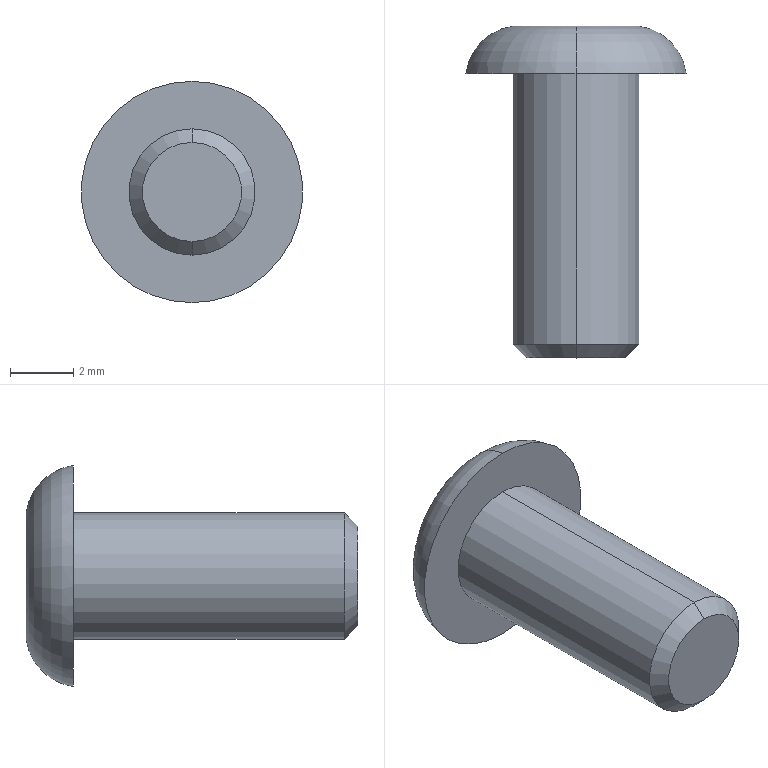Part | SolidWorks | features BaseBody 1 | 1 solid | 16 faces | box 7 x 10.5 x 7 mm | volume 150.453 mm3 | plane 10 | torus 2 | cylinder 2 | cone 2 | commonest cylinder face diameters 4 x2
STEP:
#1=CARTESIAN_POINT('',(17.5,27.,-23.5));
#2=VERTEX_POINT('',#1);
#3=CARTESIAN_POINT('',(17.5,27.,-16.5));
#4=VERTEX_POINT('',#3);
#5=CARTESIAN_POINT('',(17.5,27.,-20.));
#6=DIRECTION('',(0.,-1.,0.));
#7=DIRECTION('',(0.,0.,1.));
#8=AXIS2_PLACEMENT_3D('',#5,#6,#7);
#9=CIRCLE('',#8,3.5);
#10=EDGE_CURVE('',#2,#4,#9,.T.);
#11=ORIENTED_EDGE('',*,*,#10,.F.);
#12=CARTESIAN_POINT('',(17.5,28.5,-22.));
#13=VERTEX_POINT('',#12);
#14=CARTESIAN_POINT('',(17.5,26.766,-21.766));
#15=DIRECTION('',(1.,0.,0.));
#16=DIRECTION('',(0.,0.,-1.));
#17=AXIS2_PLACEMENT_3D('',#14,#15,#16);
#18=CIRCLE('',#17,1.75);
#19=EDGE_CURVE('',#2,#13,#18,.T.);
#20=ORIENTED_EDGE('',*,*,#19,.T.);
#21=CARTESIAN_POINT('',(17.5,28.5,-18.));
#22=VERTEX_POINT('',#21);
#23=CARTESIAN_POINT('',(17.5,28.5,-20.));
#24=DIRECTION('',(0.,-1.,0.));
#25=DIRECTION('',(0.,0.,1.));
#26=AXIS2_PLACEMENT_3D('',#23,#24,#25);
#27=CIRCLE('',#26,2.);
#28=EDGE_CURVE('',#13,#22,#27,.T.);
#29=ORIENTED_EDGE('',*,*,#28,.T.);
#30=CARTESIAN_POINT('',(17.5,26.766,-18.234));
#31=DIRECTION('',(-1.,0.,0.));
#32=DIRECTION('',(0.,-1.,0.));
#33=AXIS2_PLACEMENT_3D('',#30,#31,#32);
#34=CIRCLE('',#33,1.75);
#35=EDGE_CURVE('',#4,#22,#34,.T.);
#36=ORIENTED_EDGE('',*,*,#35,.F.);
#37=EDGE_LOOP('',(#11,#20,#29,#36));
#38=FACE_OUTER_BOUND('',#37,.T.);
#39=CARTESIAN_POINT('',(17.5,26.766,-20.));
#40=DIRECTION('',(0.,1.,0.));
#41=DIRECTION('',(0.,0.,1.));
#42=AXIS2_PLACEMENT_3D('',#39,#40,#41);
#43=TOROIDAL_SURFACE('',#42,1.766,1.75);
#44=ADVANCED_FACE('',(#38),#43,.T.);
#45=CARTESIAN_POINT('',(17.5,27.,-22.));
#46=VERTEX_POINT('',#45);
#47=CARTESIAN_POINT('',(17.5,27.,-18.));
#48=VERTEX_POINT('',#47);
#49=CARTESIAN_POINT('',(17.5,27.,-20.));
#50=DIRECTION('',(0.,-1.,0.));
#51=DIRECTION('',(0.,0.,-1.));
#52=AXIS2_PLACEMENT_3D('',#49,#50,#51);
#53=CIRCLE('',#52,2.);
#54=EDGE_CURVE('',#46,#48,#53,.T.);
#55=ORIENTED_EDGE('',*,*,#54,.T.);
#56=CARTESIAN_POINT('',(17.5,18.43,-18.));
#57=VERTEX_POINT('',#56);
#58=CARTESIAN_POINT('',(17.5,22.715,-18.));
#59=DIRECTION('',(0.,-1.,0.));
#60=VECTOR('',#59,1000.);
#61=LINE('',#58,#60);
#62=EDGE_CURVE('',#48,#57,#61,.T.);
#63=ORIENTED_EDGE('',*,*,#62,.T.);
#64=CARTESIAN_POINT('',(17.5,18.43,-22.));
#65=VERTEX_POINT('',#64);
#66=CARTESIAN_POINT('',(17.5,18.43,-20.));
#67=DIRECTION('',(0.,1.,0.));
#68=DIRECTION('',(0.,0.,-1.));
#69=AXIS2_PLACEMENT_3D('',#66,#67,#68);
#70=CIRCLE('',#69,2.);
#71=EDGE_CURVE('',#57,#65,#70,.T.);
#72=ORIENTED_EDGE('',*,*,#71,.T.);
#73=CARTESIAN_POINT('',(17.5,22.715,-22.));
#74=DIRECTION('',(0.,-1.,0.));
#75=VECTOR('',#74,1000.);
#76=LINE('',#73,#75);
#77=EDGE_CURVE('',#46,#65,#76,.T.);
#78=ORIENTED_EDGE('',*,*,#77,.F.);
#79=EDGE_LOOP('',(#55,#63,#72,#78));
#80=FACE_OUTER_BOUND('',#79,.T.);
#81=CARTESIAN_POINT('',(17.5,22.715,-20.));
#82=DIRECTION('',(0.,-1.,0.));
#83=DIRECTION('',(0.,0.,-1.));
#84=AXIS2_PLACEMENT_3D('',#81,#82,#83);
#85=CYLINDRICAL_SURFACE('',#84,2.);
#86=ADVANCED_FACE('',(#80),#85,.T.);
#87=CARTESIAN_POINT('',(17.5,18.,-18.43));
#88=VERTEX_POINT('',#87);
#89=CARTESIAN_POINT('',(17.5,18.,-21.57));
#90=VERTEX_POINT('',#89);
#91=CARTESIAN_POINT('',(17.5,18.,-20.));
#92=DIRECTION('',(0.,1.,0.));
#93=DIRECTION('',(0.,0.,1.));
#94=AXIS2_PLACEMENT_3D('',#91,#92,#93);
#95=CIRCLE('',#94,1.57);
#96=EDGE_CURVE('',#88,#90,#95,.T.);
#97=ORIENTED_EDGE('',*,*,#96,.T.);
#98=CARTESIAN_POINT('',(17.5,18.43,-22.));
#99=DIRECTION('',(0.,0.7071,-0.7071));
#100=VECTOR('',#99,1000.);
#101=LINE('',#98,#100);
#102=EDGE_CURVE('',#90,#65,#101,.T.);
#103=ORIENTED_EDGE('',*,*,#102,.T.);
#104=ORIENTED_EDGE('',*,*,#71,.F.);
#105=CARTESIAN_POINT('',(17.5,18.43,-18.));
#106=DIRECTION('',(0.,0.7071,0.7071));
#107=VECTOR('',#106,1000.);
#108=LINE('',#105,#107);
#109=EDGE_CURVE('',#88,#57,#108,.T.);
#110=ORIENTED_EDGE('',*,*,#109,.F.);
#111=EDGE_LOOP('',(#97,#103,#104,#110));
#112=FACE_OUTER_BOUND('',#111,.T.);
#113=CARTESIAN_POINT('',(17.5,18.43,-20.));
#114=DIRECTION('',(0.,1.,0.));
#115=DIRECTION('',(0.,0.,1.));
#116=AXIS2_PLACEMENT_3D('',#113,#114,#115);
#117=CONICAL_SURFACE('',#116,2.,0.7854);
#118=ADVANCED_FACE('',(#112),#117,.T.);
#119=CARTESIAN_POINT('',(17.5,27.5,-21.684));
#120=VERTEX_POINT('',#119);
#121=CARTESIAN_POINT('',(16.042,27.5,-20.842));
#122=VERTEX_POINT('',#121);
#123=CARTESIAN_POINT('',(17.5,27.5,-21.684));
#124=DIRECTION('',(-0.866,0.,0.5));
#125=VECTOR('',#124,1000.);
#126=LINE('',#123,#125);
#127=EDGE_CURVE('',#120,#122,#126,.T.);
#128=ORIENTED_EDGE('',*,*,#127,.T.);
#129=CARTESIAN_POINT('',(16.042,27.5,-19.158));
#130=VERTEX_POINT('',#129);
#131=CARTESIAN_POINT('',(16.042,27.5,-20.842));
#132=DIRECTION('',(0.,0.,1.));
#133=VECTOR('',#132,1000.);
#134=LINE('',#131,#133);
#135=EDGE_CURVE('',#122,#130,#134,.T.);
#136=ORIENTED_EDGE('',*,*,#135,.T.);
#137=CARTESIAN_POINT('',(17.5,27.5,-18.316));
#138=VERTEX_POINT('',#137);
#139=CARTESIAN_POINT('',(16.042,27.5,-19.158));
#140=DIRECTION('',(0.866,0.,0.5));
#141=VECTOR('',#140,1000.);
#142=LINE('',#139,#141);
#143=EDGE_CURVE('',#130,#138,#142,.T.);
#144=ORIENTED_EDGE('',*,*,#143,.T.);
#145=CARTESIAN_POINT('',(18.958,27.5,-19.158));
#146=VERTEX_POINT('',#145);
#147=CARTESIAN_POINT('',(17.5,27.5,-18.316));
#148=DIRECTION('',(0.866,0.,-0.5));
#149=VECTOR('',#148,1000.);
#150=LINE('',#147,#149);
#151=EDGE_CURVE('',#138,#146,#150,.T.);
#152=ORIENTED_EDGE('',*,*,#151,.T.);
#153=CARTESIAN_POINT('',(18.958,27.5,-20.842));
#154=VERTEX_POINT('',#153);
#155=CARTESIAN_POINT('',(18.958,27.5,-19.158));
#156=DIRECTION('',(0.,0.,-1.));
#157=VECTOR('',#156,1000.);
#158=LINE('',#155,#157);
#159=EDGE_CURVE('',#146,#154,#158,.T.);
#160=ORIENTED_EDGE('',*,*,#159,.T.);
#161=CARTESIAN_POINT('',(18.958,27.5,-20.842));
#162=DIRECTION('',(-0.866,0.,-0.5));
#163=VECTOR('',#162,1000.);
#164=LINE('',#161,#163);
#165=EDGE_CURVE('',#154,#120,#164,.T.);
#166=ORIENTED_EDGE('',*,*,#165,.T.);
#167=EDGE_LOOP('',(#128,#136,#144,#152,#160,#166));
#168=FACE_OUTER_BOUND('',#167,.T.);
#169=CARTESIAN_POINT('',(17.5,27.5,-20.));
#170=DIRECTION('',(0.,1.,0.));
#171=DIRECTION('',(1.,0.,0.));
#172=AXIS2_PLACEMENT_3D('',#169,#170,#171);
#173=PLANE('',#172);
#174=ADVANCED_FACE('',(#168),#173,.T.);
#175=CARTESIAN_POINT('',(16.042,28.5,-19.158));
#176=VERTEX_POINT('',#175);
#177=CARTESIAN_POINT('',(16.042,28.5,-19.158));
#178=DIRECTION('',(0.,1.,0.));
#179=VECTOR('',#178,1000.);
#180=LINE('',#177,#179);
#181=EDGE_CURVE('',#130,#176,#180,.T.);
#182=ORIENTED_EDGE('',*,*,#181,.T.);
#183=CARTESIAN_POINT('',(17.5,28.5,-18.316));
#184=VERTEX_POINT('',#183);
#185=CARTESIAN_POINT('',(17.5,28.5,-18.316));
#186=DIRECTION('',(-0.866,0.,-0.5));
#187=VECTOR('',#186,1000.);
#188=LINE('',#185,#187);
#189=EDGE_CURVE('',#184,#176,#188,.T.);
#190=ORIENTED_EDGE('',*,*,#189,.F.);
#191=CARTESIAN_POINT('',(17.5,28.5,-18.316));
#192=DIRECTION('',(0.,-1.,0.));
#193=VECTOR('',#192,1000.);
#194=LINE('',#191,#193);
#195=EDGE_CURVE('',#184,#138,#194,.T.);
#196=ORIENTED_EDGE('',*,*,#195,.T.);
#197=ORIENTED_EDGE('',*,*,#143,.F.);
#198=EDGE_LOOP('',(#182,#190,#196,#197));
#199=FACE_OUTER_BOUND('',#198,.T.);
#200=CARTESIAN_POINT('',(16.042,28.5,-19.158));
#201=DIRECTION('',(-0.5,0.,0.866));
#202=DIRECTION('',(0.,1.,0.));
#203=AXIS2_PLACEMENT_3D('',#200,#201,#202);
#204=PLANE('',#203);
#205=ADVANCED_FACE('',(#199),#204,.F.);
#206=CARTESIAN_POINT('',(16.042,28.5,-20.842));
#207=VERTEX_POINT('',#206);
#208=CARTESIAN_POINT('',(16.042,28.5,-20.842));
#209=DIRECTION('',(0.,1.,0.));
#210=VECTOR('',#209,1000.);
#211=LINE('',#208,#210);
#212=EDGE_CURVE('',#122,#207,#211,.T.);
#213=ORIENTED_EDGE('',*,*,#212,.T.);
#214=CARTESIAN_POINT('',(16.042,28.5,-21.));
#215=DIRECTION('',(0.,0.,-1.));
#216=VECTOR('',#215,1000.);
#217=LINE('',#214,#216);
#218=EDGE_CURVE('',#176,#207,#217,.T.);
#219=ORIENTED_EDGE('',*,*,#218,.F.);
#220=ORIENTED_EDGE('',*,*,#181,.F.);
#221=ORIENTED_EDGE('',*,*,#135,.F.);
#222=EDGE_LOOP('',(#213,#219,#220,#221));
#223=FACE_OUTER_BOUND('',#222,.T.);
#224=CARTESIAN_POINT('',(16.042,28.5,-20.842));
#225=DIRECTION('',(-1.,0.,0.));
#226=DIRECTION('',(0.,0.,1.));
#227=AXIS2_PLACEMENT_3D('',#224,#225,#226);
#228=PLANE('',#227);
#229=ADVANCED_FACE('',(#223),#228,.F.);
#230=CARTESIAN_POINT('',(17.5,28.5,-21.684));
#231=VERTEX_POINT('',#230);
#232=CARTESIAN_POINT('',(17.5,28.5,-21.684));
#233=DIRECTION('',(0.,1.,0.));
#234=VECTOR('',#233,1000.);
#235=LINE('',#232,#234);
#236=EDGE_CURVE('',#120,#231,#235,.T.);
#237=ORIENTED_EDGE('',*,*,#236,.T.);
#238=CARTESIAN_POINT('',(16.042,28.5,-20.842));
#239=DIRECTION('',(0.866,0.,-0.5));
#240=VECTOR('',#239,1000.);
#241=LINE('',#238,#240);
#242=EDGE_CURVE('',#207,#231,#241,.T.);
#243=ORIENTED_EDGE('',*,*,#242,.F.);
#244=ORIENTED_EDGE('',*,*,#212,.F.);
#245=ORIENTED_EDGE('',*,*,#127,.F.);
#246=EDGE_LOOP('',(#237,#243,#244,#245));
#247=FACE_OUTER_BOUND('',#246,.T.);
#248=CARTESIAN_POINT('',(17.5,28.5,-21.684));
#249=DIRECTION('',(-0.5,0.,-0.866));
#250=DIRECTION('',(-0.866,0.,0.5));
#251=AXIS2_PLACEMENT_3D('',#248,#249,#250);
#252=PLANE('',#251);
#253=ADVANCED_FACE('',(#247),#252,.F.);
#254=CARTESIAN_POINT('',(18.958,28.5,-20.842));
#255=VERTEX_POINT('',#254);
#256=CARTESIAN_POINT('',(18.958,28.5,-20.842));
#257=DIRECTION('',(0.,1.,0.));
#258=VECTOR('',#257,1000.);
#259=LINE('',#256,#258);
#260=EDGE_CURVE('',#154,#255,#259,.T.);
#261=ORIENTED_EDGE('',*,*,#260,.T.);
#262=CARTESIAN_POINT('',(17.5,28.5,-21.684));
#263=DIRECTION('',(0.866,0.,0.5));
#264=VECTOR('',#263,1000.);
#265=LINE('',#262,#264);
#266=EDGE_CURVE('',#231,#255,#265,.T.);
#267=ORIENTED_EDGE('',*,*,#266,.F.);
#268=ORIENTED_EDGE('',*,*,#236,.F.);
#269=ORIENTED_EDGE('',*,*,#165,.F.);
#270=EDGE_LOOP('',(#261,#267,#268,#269));
#271=FACE_OUTER_BOUND('',#270,.T.);
#272=CARTESIAN_POINT('',(18.958,28.5,-20.842));
#273=DIRECTION('',(0.5,0.,-0.866));
#274=DIRECTION('',(0.,-1.,0.));
#275=AXIS2_PLACEMENT_3D('',#272,#273,#274);
#276=PLANE('',#275);
#277=ADVANCED_FACE('',(#271),#276,.F.);
#278=CARTESIAN_POINT('',(18.958,28.5,-19.158));
#279=VERTEX_POINT('',#278);
#280=CARTESIAN_POINT('',(18.958,28.5,-19.158));
#281=DIRECTION('',(0.,1.,0.));
#282=VECTOR('',#281,1000.);
#283=LINE('',#280,#282);
#284=EDGE_CURVE('',#146,#279,#283,.T.);
#285=ORIENTED_EDGE('',*,*,#284,.T.);
#286=CARTESIAN_POINT('',(18.958,28.5,-21.));
#287=DIRECTION('',(0.,0.,1.));
#288=VECTOR('',#287,1000.);
#289=LINE('',#286,#288);
#290=EDGE_CURVE('',#255,#279,#289,.T.);
#291=ORIENTED_EDGE('',*,*,#290,.F.);
#292=ORIENTED_EDGE('',*,*,#260,.F.);
#293=ORIENTED_EDGE('',*,*,#159,.F.);
#294=EDGE_LOOP('',(#285,#291,#292,#293));
#295=FACE_OUTER_BOUND('',#294,.T.);
#296=CARTESIAN_POINT('',(18.958,28.5,-19.158));
#297=DIRECTION('',(1.,0.,0.));
#298=DIRECTION('',(0.,1.,0.));
#299=AXIS2_PLACEMENT_3D('',#296,#297,#298);
#300=PLANE('',#299);
#301=ADVANCED_FACE('',(#295),#300,.F.);
#302=ORIENTED_EDGE('',*,*,#195,.F.);
#303=CARTESIAN_POINT('',(18.958,28.5,-19.158));
#304=DIRECTION('',(-0.866,0.,0.5));
#305=VECTOR('',#304,1000.);
#306=LINE('',#303,#305);
#307=EDGE_CURVE('',#279,#184,#306,.T.);
#308=ORIENTED_EDGE('',*,*,#307,.F.);
#309=ORIENTED_EDGE('',*,*,#284,.F.);
#310=ORIENTED_EDGE('',*,*,#151,.F.);
#311=EDGE_LOOP('',(#302,#308,#309,#310));
#312=FACE_OUTER_BOUND('',#311,.T.);
#313=CARTESIAN_POINT('',(17.5,28.5,-18.316));
#314=DIRECTION('',(0.5,0.,0.866));
#315=DIRECTION('',(0.,-1.,0.));
#316=AXIS2_PLACEMENT_3D('',#313,#314,#315);
#317=PLANE('',#316);
#318=ADVANCED_FACE('',(#312),#317,.F.);
#319=ORIENTED_EDGE('',*,*,#290,.T.);
#320=ORIENTED_EDGE('',*,*,#307,.T.);
#321=ORIENTED_EDGE('',*,*,#189,.T.);
#322=ORIENTED_EDGE('',*,*,#218,.T.);
#323=ORIENTED_EDGE('',*,*,#242,.T.);
#324=ORIENTED_EDGE('',*,*,#266,.T.);
#325=EDGE_LOOP('',(#319,#320,#321,#322,#323,#324));
#326=FACE_BOUND('',#325,.T.);
#327=CARTESIAN_POINT('',(17.5,28.5,-20.));
#328=DIRECTION('',(0.,-1.,0.));
#329=DIRECTION('',(0.,0.,1.));
#330=AXIS2_PLACEMENT_3D('',#327,#328,#329);
#331=CIRCLE('',#330,2.);
#332=EDGE_CURVE('',#22,#13,#331,.T.);
#333=ORIENTED_EDGE('',*,*,#332,.F.);
#334=ORIENTED_EDGE('',*,*,#28,.F.);
#335=EDGE_LOOP('',(#333,#334));
#336=FACE_OUTER_BOUND('',#335,.T.);
#337=CARTESIAN_POINT('',(17.5,28.5,-21.));
#338=DIRECTION('',(0.,1.,0.));
#339=DIRECTION('',(1.,0.,0.));
#340=AXIS2_PLACEMENT_3D('',#337,#338,#339);
#341=PLANE('',#340);
#342=ADVANCED_FACE('',(#326,#336),#341,.T.);
#343=ORIENTED_EDGE('',*,*,#96,.F.);
#344=CARTESIAN_POINT('',(17.5,18.,-20.));
#345=DIRECTION('',(0.,1.,0.));
#346=DIRECTION('',(0.,0.,1.));
#347=AXIS2_PLACEMENT_3D('',#344,#345,#346);
#348=CIRCLE('',#347,1.57);
#349=EDGE_CURVE('',#90,#88,#348,.T.);
#350=ORIENTED_EDGE('',*,*,#349,.F.);
#351=EDGE_LOOP('',(#343,#350));
#352=FACE_OUTER_BOUND('',#351,.T.);
#353=CARTESIAN_POINT('',(17.5,18.,-20.785));
#354=DIRECTION('',(0.,-1.,0.));
#355=DIRECTION('',(0.,0.,-1.));
#356=AXIS2_PLACEMENT_3D('',#353,#354,#355);
#357=PLANE('',#356);
#358=ADVANCED_FACE('',(#352),#357,.T.);
#359=ORIENTED_EDGE('',*,*,#54,.F.);
#360=CARTESIAN_POINT('',(17.5,27.,-20.));
#361=DIRECTION('',(0.,-1.,0.));
#362=DIRECTION('',(0.,0.,-1.));
#363=AXIS2_PLACEMENT_3D('',#360,#361,#362);
#364=CIRCLE('',#363,2.);
#365=EDGE_CURVE('',#48,#46,#364,.T.);
#366=ORIENTED_EDGE('',*,*,#365,.F.);
#367=EDGE_LOOP('',(#359,#366));
#368=FACE_BOUND('',#367,.T.);
#369=CARTESIAN_POINT('',(17.5,27.,-20.));
#370=DIRECTION('',(0.,-1.,0.));
#371=DIRECTION('',(0.,0.,1.));
#372=AXIS2_PLACEMENT_3D('',#369,#370,#371);
#373=CIRCLE('',#372,3.5);
#374=EDGE_CURVE('',#4,#2,#373,.T.);
#375=ORIENTED_EDGE('',*,*,#374,.T.);
#376=ORIENTED_EDGE('',*,*,#10,.T.);
#377=EDGE_LOOP('',(#375,#376));
#378=FACE_OUTER_BOUND('',#377,.T.);
#379=CARTESIAN_POINT('',(17.5,27.,-22.75));
#380=DIRECTION('',(0.,-1.,0.));
#381=DIRECTION('',(-1.,0.,0.));
#382=AXIS2_PLACEMENT_3D('',#379,#380,#381);
#383=PLANE('',#382);
#384=ADVANCED_FACE('',(#368,#378),#383,.T.);
#385=ORIENTED_EDGE('',*,*,#102,.F.);
#386=ORIENTED_EDGE('',*,*,#349,.T.);
#387=ORIENTED_EDGE('',*,*,#109,.T.);
#388=CARTESIAN_POINT('',(17.5,18.43,-20.));
#389=DIRECTION('',(0.,1.,0.));
#390=DIRECTION('',(0.,0.,-1.));
#391=AXIS2_PLACEMENT_3D('',#388,#389,#390);
#392=CIRCLE('',#391,2.);
#393=EDGE_CURVE('',#65,#57,#392,.T.);
#394=ORIENTED_EDGE('',*,*,#393,.F.);
#395=EDGE_LOOP('',(#385,#386,#387,#394));
#396=FACE_OUTER_BOUND('',#395,.T.);
#397=CARTESIAN_POINT('',(17.5,18.43,-20.));
#398=DIRECTION('',(0.,1.,0.));
#399=DIRECTION('',(0.,0.,1.));
#400=AXIS2_PLACEMENT_3D('',#397,#398,#399);
#401=CONICAL_SURFACE('',#400,2.,0.7854);
#402=ADVANCED_FACE('',(#396),#401,.T.);
#403=ORIENTED_EDGE('',*,*,#62,.F.);
#404=ORIENTED_EDGE('',*,*,#365,.T.);
#405=ORIENTED_EDGE('',*,*,#77,.T.);
#406=ORIENTED_EDGE('',*,*,#393,.T.);
#407=EDGE_LOOP('',(#403,#404,#405,#406));
#408=FACE_OUTER_BOUND('',#407,.T.);
#409=CARTESIAN_POINT('',(17.5,22.715,-20.));
#410=DIRECTION('',(0.,-1.,0.));
#411=DIRECTION('',(0.,0.,-1.));
#412=AXIS2_PLACEMENT_3D('',#409,#410,#411);
#413=CYLINDRICAL_SURFACE('',#412,2.);
#414=ADVANCED_FACE('',(#408),#413,.T.);
#415=ORIENTED_EDGE('',*,*,#19,.F.);
#416=ORIENTED_EDGE('',*,*,#374,.F.);
#417=ORIENTED_EDGE('',*,*,#35,.T.);
#418=ORIENTED_EDGE('',*,*,#332,.T.);
#419=EDGE_LOOP('',(#415,#416,#417,#418));
#420=FACE_OUTER_BOUND('',#419,.T.);
#421=CARTESIAN_POINT('',(17.5,26.766,-20.));
#422=DIRECTION('',(0.,1.,0.));
#423=DIRECTION('',(0.,0.,1.));
#424=AXIS2_PLACEMENT_3D('',#421,#422,#423);
#425=TOROIDAL_SURFACE('',#424,1.766,1.75);
#426=ADVANCED_FACE('',(#420),#425,.T.);
#427=CLOSED_SHELL('',(#44,#86,#118,#174,#205,#229,#253,#277,#301,#318,#342,#358,#384,#402,#414,#426));
#428=MANIFOLD_SOLID_BREP('',#427);
#429=CARTESIAN_POINT('',(0.,0.,0.));
#430=DIRECTION('',(0.,0.,1.));
#431=DIRECTION('',(1.,0.,0.));
#432=AXIS2_PLACEMENT_3D('',#429,#430,#431);
#433=(LENGTH_UNIT()NAMED_UNIT(*)SI_UNIT(.MILLI.,.METRE.));
#434=UNCERTAINTY_MEASURE_WITH_UNIT(LENGTH_MEASURE(0.00001),#433,'','');
#435=(NAMED_UNIT(*)PLANE_ANGLE_UNIT()SI_UNIT($,.RADIAN.));
#436=(NAMED_UNIT(*)SI_UNIT($,.STERADIAN.)SOLID_ANGLE_UNIT());
#437=(GEOMETRIC_REPRESENTATION_CONTEXT(3)GLOBAL_UNCERTAINTY_ASSIGNED_CONTEXT((#434))GLOBAL_UNIT_ASSIGNED_CONTEXT((#433,#435,#436))REPRESENTATION_CONTEXT('',''));
#438=ADVANCED_BREP_SHAPE_REPRESENTATION('',(#428,#432),#437);